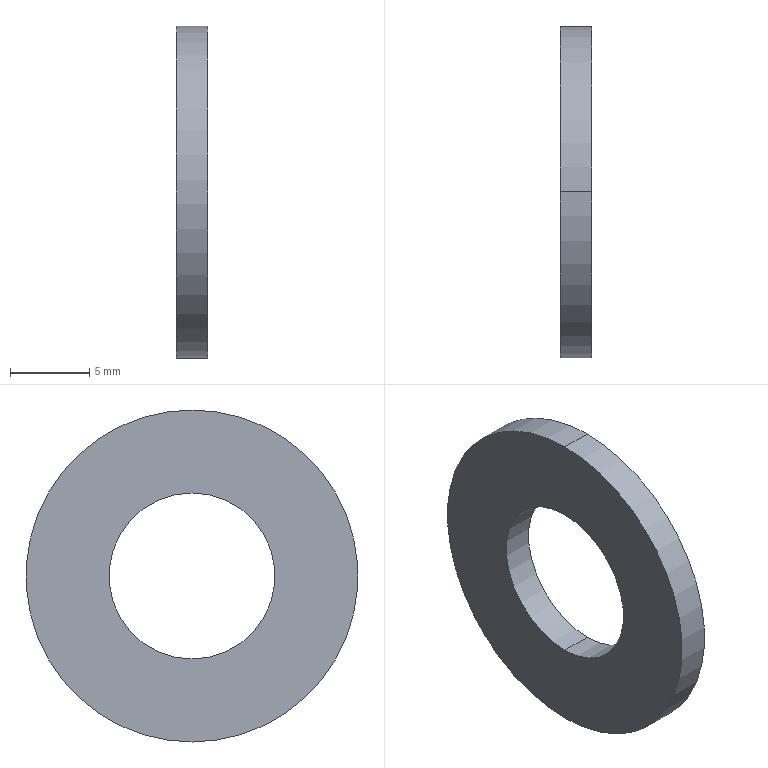Part | STEP file | 0229_316_SPWF10 | 1 solid | 6 faces | box 2 x 21 x 21 mm | volume 519.541 mm3 | cylinder 4 | plane 2 | commonest cylinder face diameters 10.5 x2 21 x2
STEP:
#1=CARTESIAN_POINT('',(0.,0.,0.));
#2=DIRECTION('',(0.,0.,1.));
#3=DIRECTION('',(1.,0.,0.));
#4=AXIS2_PLACEMENT_3D('',#1,#2,#3);
#5=CARTESIAN_POINT('',(-1.,0.,10.5));
#6=VERTEX_POINT('',#5);
#7=CARTESIAN_POINT('',(-1.,0.,-10.5));
#8=VERTEX_POINT('',#7);
#9=CARTESIAN_POINT('',(-1.,0.,0.));
#10=DIRECTION('',(-1.,0.,0.));
#11=DIRECTION('',(0.,0.,-1.));
#12=AXIS2_PLACEMENT_3D('',#9,#10,#11);
#13=CIRCLE('',#12,10.5);
#14=CARTESIAN_POINT('',(0.,0.,0.));
#15=DIRECTION('',(1.,0.,0.));
#16=DIRECTION('',(0.,0.,-1.));
#17=AXIS2_PLACEMENT_3D('',#14,#15,#16);
#18=CYLINDRICAL_SURFACE('',#17,10.5);
#19=CARTESIAN_POINT('',(6.283,-1.));
#20=DIRECTION('',(-1.,0.));
#21=VECTOR('',#20,1.);
#22=LINE('',#19,#21);
#23=(GEOMETRIC_REPRESENTATION_CONTEXT(2)PARAMETRIC_REPRESENTATION_CONTEXT()REPRESENTATION_CONTEXT('',''));
#24=DEFINITIONAL_REPRESENTATION('',(#22),#23);
#25=PCURVE('',#18,#24);
#26=CARTESIAN_POINT('',(-1.,7.875,0.));
#27=DIRECTION('',(-1.,0.,0.));
#28=DIRECTION('',(0.,0.,1.));
#29=AXIS2_PLACEMENT_3D('',#26,#27,#28);
#30=PLANE('',#29);
#31=CARTESIAN_POINT('',(0.,-7.875));
#32=DIRECTION('',(-1.,0.));
#33=AXIS2_PLACEMENT_2D('',#31,#32);
#34=CIRCLE('',#33,10.5);
#35=(GEOMETRIC_REPRESENTATION_CONTEXT(2)PARAMETRIC_REPRESENTATION_CONTEXT()REPRESENTATION_CONTEXT('',''));
#36=DEFINITIONAL_REPRESENTATION('',(#34),#35);
#37=PCURVE('',#30,#36);
#38=SURFACE_CURVE('',#13,(#25,#37),.PCURVE_S1.);
#39=EDGE_CURVE('',#6,#8,#38,.T.);
#40=ORIENTED_EDGE('',*,*,#39,.F.);
#41=CARTESIAN_POINT('',(1.,0.,10.5));
#42=VERTEX_POINT('',#41);
#43=CARTESIAN_POINT('',(0.,0.,10.5));
#44=DIRECTION('',(1.,0.,0.));
#45=VECTOR('',#44,1.);
#46=LINE('',#43,#45);
#47=CARTESIAN_POINT('',(3.142,0.));
#48=DIRECTION('',(0.,1.));
#49=VECTOR('',#48,1.);
#50=LINE('',#47,#49);
#51=(GEOMETRIC_REPRESENTATION_CONTEXT(2)PARAMETRIC_REPRESENTATION_CONTEXT()REPRESENTATION_CONTEXT('',''));
#52=DEFINITIONAL_REPRESENTATION('',(#50),#51);
#53=PCURVE('',#18,#52);
#54=CARTESIAN_POINT('',(0.,0.,0.));
#55=DIRECTION('',(1.,0.,0.));
#56=DIRECTION('',(0.,0.,-1.));
#57=AXIS2_PLACEMENT_3D('',#54,#55,#56);
#58=CYLINDRICAL_SURFACE('',#57,10.5);
#59=CARTESIAN_POINT('',(3.142,0.));
#60=DIRECTION('',(0.,1.));
#61=VECTOR('',#60,1.);
#62=LINE('',#59,#61);
#63=(GEOMETRIC_REPRESENTATION_CONTEXT(2)PARAMETRIC_REPRESENTATION_CONTEXT()REPRESENTATION_CONTEXT('',''));
#64=DEFINITIONAL_REPRESENTATION('',(#62),#63);
#65=PCURVE('',#58,#64);
#66=SURFACE_CURVE('',#46,(#53,#65),.PCURVE_S1.);
#67=EDGE_CURVE('',#6,#42,#66,.T.);
#68=ORIENTED_EDGE('',*,*,#67,.T.);
#69=CARTESIAN_POINT('',(1.,0.,-10.5));
#70=VERTEX_POINT('',#69);
#71=CARTESIAN_POINT('',(1.,0.,0.));
#72=DIRECTION('',(-1.,0.,0.));
#73=DIRECTION('',(0.,0.,-1.));
#74=AXIS2_PLACEMENT_3D('',#71,#72,#73);
#75=CIRCLE('',#74,10.5);
#76=CARTESIAN_POINT('',(6.283,1.));
#77=DIRECTION('',(-1.,0.));
#78=VECTOR('',#77,1.);
#79=LINE('',#76,#78);
#80=(GEOMETRIC_REPRESENTATION_CONTEXT(2)PARAMETRIC_REPRESENTATION_CONTEXT()REPRESENTATION_CONTEXT('',''));
#81=DEFINITIONAL_REPRESENTATION('',(#79),#80);
#82=PCURVE('',#18,#81);
#83=CARTESIAN_POINT('',(1.,7.875,0.));
#84=DIRECTION('',(1.,0.,0.));
#85=DIRECTION('',(0.,0.,-1.));
#86=AXIS2_PLACEMENT_3D('',#83,#84,#85);
#87=PLANE('',#86);
#88=CARTESIAN_POINT('',(10.5,-7.875));
#89=CARTESIAN_POINT('',(10.5,-26.062));
#90=CARTESIAN_POINT('',(-5.25,-16.968));
#91=CARTESIAN_POINT('',(-21.,-7.875));
#92=CARTESIAN_POINT('',(-5.25,1.218));
#93=CARTESIAN_POINT('',(10.5,10.312));
#94=CARTESIAN_POINT('',(10.5,-7.875));
#95=(BOUNDED_CURVE()B_SPLINE_CURVE(2,(#88,#89,#90,#91,#92,#93,#94),.UNSPECIFIED.,.T.,.F.)B_SPLINE_CURVE_WITH_KNOTS((1,2,2,2,2,1),(-2.094,0.,2.094,4.189,6.283,8.378),.UNSPECIFIED.)CURVE()GEOMETRIC_REPRESENTATION_ITEM()RATIONAL_B_SPLINE_CURVE((1.,0.5,1.,0.5,1.,0.5,1.))REPRESENTATION_ITEM(''));
#96=(GEOMETRIC_REPRESENTATION_CONTEXT(2)PARAMETRIC_REPRESENTATION_CONTEXT()REPRESENTATION_CONTEXT('',''));
#97=DEFINITIONAL_REPRESENTATION('',(#95),#96);
#98=PCURVE('',#87,#97);
#99=SURFACE_CURVE('',#75,(#82,#98),.PCURVE_S1.);
#100=EDGE_CURVE('',#42,#70,#99,.T.);
#101=ORIENTED_EDGE('',*,*,#100,.T.);
#102=CARTESIAN_POINT('',(0.,0.,-10.5));
#103=DIRECTION('',(1.,0.,0.));
#104=VECTOR('',#103,1.);
#105=LINE('',#102,#104);
#106=CARTESIAN_POINT('',(0.,0.));
#107=DIRECTION('',(0.,1.));
#108=VECTOR('',#107,1.);
#109=LINE('',#106,#108);
#110=(GEOMETRIC_REPRESENTATION_CONTEXT(2)PARAMETRIC_REPRESENTATION_CONTEXT()REPRESENTATION_CONTEXT('',''));
#111=DEFINITIONAL_REPRESENTATION('',(#109),#110);
#112=PCURVE('',#18,#111);
#113=CARTESIAN_POINT('',(6.283,0.));
#114=DIRECTION('',(0.,1.));
#115=VECTOR('',#114,1.);
#116=LINE('',#113,#115);
#117=(GEOMETRIC_REPRESENTATION_CONTEXT(2)PARAMETRIC_REPRESENTATION_CONTEXT()REPRESENTATION_CONTEXT('',''));
#118=DEFINITIONAL_REPRESENTATION('',(#116),#117);
#119=PCURVE('',#58,#118);
#120=SURFACE_CURVE('',#105,(#112,#119),.PCURVE_S1.);
#121=EDGE_CURVE('',#8,#70,#120,.T.);
#122=ORIENTED_EDGE('',*,*,#121,.F.);
#123=EDGE_LOOP('',(#40,#68,#101,#122));
#124=FACE_BOUND('',#123,.T.);
#125=ADVANCED_FACE('',(#124),#18,.T.);
#126=CARTESIAN_POINT('',(-1.,0.,-5.25));
#127=VERTEX_POINT('',#126);
#128=CARTESIAN_POINT('',(1.,0.,-5.25));
#129=VERTEX_POINT('',#128);
#130=CARTESIAN_POINT('',(0.,0.,-5.25));
#131=DIRECTION('',(1.,0.,0.));
#132=VECTOR('',#131,1.);
#133=LINE('',#130,#132);
#134=CARTESIAN_POINT('',(0.,0.,0.));
#135=DIRECTION('',(1.,0.,0.));
#136=DIRECTION('',(0.,0.,-1.));
#137=AXIS2_PLACEMENT_3D('',#134,#135,#136);
#138=CYLINDRICAL_SURFACE('',#137,5.25);
#139=CARTESIAN_POINT('',(6.283,0.));
#140=DIRECTION('',(0.,1.));
#141=VECTOR('',#140,1.);
#142=LINE('',#139,#141);
#143=(GEOMETRIC_REPRESENTATION_CONTEXT(2)PARAMETRIC_REPRESENTATION_CONTEXT()REPRESENTATION_CONTEXT('',''));
#144=DEFINITIONAL_REPRESENTATION('',(#142),#143);
#145=PCURVE('',#138,#144);
#146=CARTESIAN_POINT('',(0.,0.,0.));
#147=DIRECTION('',(1.,0.,0.));
#148=DIRECTION('',(0.,0.,-1.));
#149=AXIS2_PLACEMENT_3D('',#146,#147,#148);
#150=CYLINDRICAL_SURFACE('',#149,5.25);
#151=CARTESIAN_POINT('',(0.,0.));
#152=DIRECTION('',(0.,1.));
#153=VECTOR('',#152,1.);
#154=LINE('',#151,#153);
#155=(GEOMETRIC_REPRESENTATION_CONTEXT(2)PARAMETRIC_REPRESENTATION_CONTEXT()REPRESENTATION_CONTEXT('',''));
#156=DEFINITIONAL_REPRESENTATION('',(#154),#155);
#157=PCURVE('',#150,#156);
#158=SURFACE_CURVE('',#133,(#145,#157),.PCURVE_S1.);
#159=EDGE_CURVE('',#127,#129,#158,.T.);
#160=ORIENTED_EDGE('',*,*,#159,.T.);
#161=CARTESIAN_POINT('',(1.,0.,5.25));
#162=VERTEX_POINT('',#161);
#163=CARTESIAN_POINT('',(1.,0.,0.));
#164=DIRECTION('',(-1.,0.,0.));
#165=DIRECTION('',(0.,0.,-1.));
#166=AXIS2_PLACEMENT_3D('',#163,#164,#165);
#167=CIRCLE('',#166,5.25);
#168=CARTESIAN_POINT('',(6.283,1.));
#169=DIRECTION('',(-1.,0.));
#170=VECTOR('',#169,1.);
#171=LINE('',#168,#170);
#172=(GEOMETRIC_REPRESENTATION_CONTEXT(2)PARAMETRIC_REPRESENTATION_CONTEXT()REPRESENTATION_CONTEXT('',''));
#173=DEFINITIONAL_REPRESENTATION('',(#171),#172);
#174=PCURVE('',#138,#173);
#175=CARTESIAN_POINT('',(5.25,-7.875));
#176=CARTESIAN_POINT('',(5.25,-16.968));
#177=CARTESIAN_POINT('',(-2.625,-12.422));
#178=CARTESIAN_POINT('',(-10.5,-7.875));
#179=CARTESIAN_POINT('',(-2.625,-3.328));
#180=CARTESIAN_POINT('',(5.25,1.218));
#181=CARTESIAN_POINT('',(5.25,-7.875));
#182=(BOUNDED_CURVE()B_SPLINE_CURVE(2,(#175,#176,#177,#178,#179,#180,#181),.UNSPECIFIED.,.T.,.F.)B_SPLINE_CURVE_WITH_KNOTS((1,2,2,2,2,1),(-2.094,0.,2.094,4.189,6.283,8.378),.UNSPECIFIED.)CURVE()GEOMETRIC_REPRESENTATION_ITEM()RATIONAL_B_SPLINE_CURVE((1.,0.5,1.,0.5,1.,0.5,1.))REPRESENTATION_ITEM(''));
#183=(GEOMETRIC_REPRESENTATION_CONTEXT(2)PARAMETRIC_REPRESENTATION_CONTEXT()REPRESENTATION_CONTEXT('',''));
#184=DEFINITIONAL_REPRESENTATION('',(#182),#183);
#185=PCURVE('',#87,#184);
#186=SURFACE_CURVE('',#167,(#174,#185),.PCURVE_S1.);
#187=EDGE_CURVE('',#129,#162,#186,.T.);
#188=ORIENTED_EDGE('',*,*,#187,.T.);
#189=CARTESIAN_POINT('',(-1.,0.,5.25));
#190=VERTEX_POINT('',#189);
#191=CARTESIAN_POINT('',(0.,0.,5.25));
#192=DIRECTION('',(1.,0.,0.));
#193=VECTOR('',#192,1.);
#194=LINE('',#191,#193);
#195=CARTESIAN_POINT('',(3.142,0.));
#196=DIRECTION('',(0.,1.));
#197=VECTOR('',#196,1.);
#198=LINE('',#195,#197);
#199=(GEOMETRIC_REPRESENTATION_CONTEXT(2)PARAMETRIC_REPRESENTATION_CONTEXT()REPRESENTATION_CONTEXT('',''));
#200=DEFINITIONAL_REPRESENTATION('',(#198),#199);
#201=PCURVE('',#138,#200);
#202=CARTESIAN_POINT('',(3.142,0.));
#203=DIRECTION('',(0.,1.));
#204=VECTOR('',#203,1.);
#205=LINE('',#202,#204);
#206=(GEOMETRIC_REPRESENTATION_CONTEXT(2)PARAMETRIC_REPRESENTATION_CONTEXT()REPRESENTATION_CONTEXT('',''));
#207=DEFINITIONAL_REPRESENTATION('',(#205),#206);
#208=PCURVE('',#150,#207);
#209=SURFACE_CURVE('',#194,(#201,#208),.PCURVE_S1.);
#210=EDGE_CURVE('',#190,#162,#209,.T.);
#211=ORIENTED_EDGE('',*,*,#210,.F.);
#212=CARTESIAN_POINT('',(-1.,0.,0.));
#213=DIRECTION('',(1.,0.,0.));
#214=DIRECTION('',(0.,0.,-1.));
#215=AXIS2_PLACEMENT_3D('',#212,#213,#214);
#216=CIRCLE('',#215,5.25);
#217=CARTESIAN_POINT('',(0.,-1.));
#218=DIRECTION('',(1.,0.));
#219=VECTOR('',#218,1.);
#220=LINE('',#217,#219);
#221=(GEOMETRIC_REPRESENTATION_CONTEXT(2)PARAMETRIC_REPRESENTATION_CONTEXT()REPRESENTATION_CONTEXT('',''));
#222=DEFINITIONAL_REPRESENTATION('',(#220),#221);
#223=PCURVE('',#138,#222);
#224=CARTESIAN_POINT('',(-5.25,-7.875));
#225=CARTESIAN_POINT('',(-5.25,1.218));
#226=CARTESIAN_POINT('',(2.625,-3.328));
#227=CARTESIAN_POINT('',(10.5,-7.875));
#228=CARTESIAN_POINT('',(2.625,-12.422));
#229=CARTESIAN_POINT('',(-5.25,-16.968));
#230=CARTESIAN_POINT('',(-5.25,-7.875));
#231=(BOUNDED_CURVE()B_SPLINE_CURVE(2,(#224,#225,#226,#227,#228,#229,#230),.UNSPECIFIED.,.T.,.F.)B_SPLINE_CURVE_WITH_KNOTS((1,2,2,2,2,1),(-2.094,0.,2.094,4.189,6.283,8.378),.UNSPECIFIED.)CURVE()GEOMETRIC_REPRESENTATION_ITEM()RATIONAL_B_SPLINE_CURVE((1.,0.5,1.,0.5,1.,0.5,1.))REPRESENTATION_ITEM(''));
#232=(GEOMETRIC_REPRESENTATION_CONTEXT(2)PARAMETRIC_REPRESENTATION_CONTEXT()REPRESENTATION_CONTEXT('',''));
#233=DEFINITIONAL_REPRESENTATION('',(#231),#232);
#234=PCURVE('',#30,#233);
#235=SURFACE_CURVE('',#216,(#223,#234),.PCURVE_S1.);
#236=EDGE_CURVE('',#190,#127,#235,.T.);
#237=ORIENTED_EDGE('',*,*,#236,.T.);
#238=EDGE_LOOP('',(#160,#188,#211,#237));
#239=FACE_BOUND('',#238,.F.);
#240=ADVANCED_FACE('',(#239),#138,.F.);
#241=CARTESIAN_POINT('',(-1.,0.,0.));
#242=DIRECTION('',(-1.,0.,0.));
#243=DIRECTION('',(0.,0.,-1.));
#244=AXIS2_PLACEMENT_3D('',#241,#242,#243);
#245=CIRCLE('',#244,10.5);
#246=CARTESIAN_POINT('',(0.,-7.875));
#247=DIRECTION('',(-1.,0.));
#248=AXIS2_PLACEMENT_2D('',#246,#247);
#249=CIRCLE('',#248,10.5);
#250=(GEOMETRIC_REPRESENTATION_CONTEXT(2)PARAMETRIC_REPRESENTATION_CONTEXT()REPRESENTATION_CONTEXT('',''));
#251=DEFINITIONAL_REPRESENTATION('',(#249),#250);
#252=PCURVE('',#30,#251);
#253=CARTESIAN_POINT('',(6.283,-1.));
#254=DIRECTION('',(-1.,0.));
#255=VECTOR('',#254,1.);
#256=LINE('',#253,#255);
#257=(GEOMETRIC_REPRESENTATION_CONTEXT(2)PARAMETRIC_REPRESENTATION_CONTEXT()REPRESENTATION_CONTEXT('',''));
#258=DEFINITIONAL_REPRESENTATION('',(#256),#257);
#259=PCURVE('',#58,#258);
#260=SURFACE_CURVE('',#245,(#252,#259),.PCURVE_S1.);
#261=EDGE_CURVE('',#8,#6,#260,.T.);
#262=ORIENTED_EDGE('',*,*,#261,.T.);
#263=ORIENTED_EDGE('',*,*,#39,.T.);
#264=EDGE_LOOP('',(#262,#263));
#265=FACE_BOUND('',#264,.T.);
#266=CARTESIAN_POINT('',(-1.,0.,0.));
#267=DIRECTION('',(1.,0.,0.));
#268=DIRECTION('',(0.,0.,-1.));
#269=AXIS2_PLACEMENT_3D('',#266,#267,#268);
#270=CIRCLE('',#269,5.25);
#271=CARTESIAN_POINT('',(-5.25,-7.875));
#272=CARTESIAN_POINT('',(-5.25,1.218));
#273=CARTESIAN_POINT('',(2.625,-3.328));
#274=CARTESIAN_POINT('',(10.5,-7.875));
#275=CARTESIAN_POINT('',(2.625,-12.422));
#276=CARTESIAN_POINT('',(-5.25,-16.968));
#277=CARTESIAN_POINT('',(-5.25,-7.875));
#278=(BOUNDED_CURVE()B_SPLINE_CURVE(2,(#271,#272,#273,#274,#275,#276,#277),.UNSPECIFIED.,.T.,.F.)B_SPLINE_CURVE_WITH_KNOTS((1,2,2,2,2,1),(-2.094,0.,2.094,4.189,6.283,8.378),.UNSPECIFIED.)CURVE()GEOMETRIC_REPRESENTATION_ITEM()RATIONAL_B_SPLINE_CURVE((1.,0.5,1.,0.5,1.,0.5,1.))REPRESENTATION_ITEM(''));
#279=(GEOMETRIC_REPRESENTATION_CONTEXT(2)PARAMETRIC_REPRESENTATION_CONTEXT()REPRESENTATION_CONTEXT('',''));
#280=DEFINITIONAL_REPRESENTATION('',(#278),#279);
#281=PCURVE('',#30,#280);
#282=CARTESIAN_POINT('',(0.,-1.));
#283=DIRECTION('',(1.,0.));
#284=VECTOR('',#283,1.);
#285=LINE('',#282,#284);
#286=(GEOMETRIC_REPRESENTATION_CONTEXT(2)PARAMETRIC_REPRESENTATION_CONTEXT()REPRESENTATION_CONTEXT('',''));
#287=DEFINITIONAL_REPRESENTATION('',(#285),#286);
#288=PCURVE('',#150,#287);
#289=SURFACE_CURVE('',#270,(#281,#288),.PCURVE_S1.);
#290=EDGE_CURVE('',#127,#190,#289,.T.);
#291=ORIENTED_EDGE('',*,*,#290,.T.);
#292=ORIENTED_EDGE('',*,*,#236,.T.);
#293=EDGE_LOOP('',(#291,#292));
#294=FACE_BOUND('',#293,.T.);
#295=ADVANCED_FACE('',(#265,#294),#30,.T.);
#296=ORIENTED_EDGE('',*,*,#67,.F.);
#297=ORIENTED_EDGE('',*,*,#261,.F.);
#298=ORIENTED_EDGE('',*,*,#121,.T.);
#299=CARTESIAN_POINT('',(1.,0.,0.));
#300=DIRECTION('',(-1.,0.,0.));
#301=DIRECTION('',(0.,0.,-1.));
#302=AXIS2_PLACEMENT_3D('',#299,#300,#301);
#303=CIRCLE('',#302,10.5);
#304=CARTESIAN_POINT('',(6.283,1.));
#305=DIRECTION('',(-1.,0.));
#306=VECTOR('',#305,1.);
#307=LINE('',#304,#306);
#308=(GEOMETRIC_REPRESENTATION_CONTEXT(2)PARAMETRIC_REPRESENTATION_CONTEXT()REPRESENTATION_CONTEXT('',''));
#309=DEFINITIONAL_REPRESENTATION('',(#307),#308);
#310=PCURVE('',#58,#309);
#311=CARTESIAN_POINT('',(10.5,-7.875));
#312=CARTESIAN_POINT('',(10.5,-26.062));
#313=CARTESIAN_POINT('',(-5.25,-16.968));
#314=CARTESIAN_POINT('',(-21.,-7.875));
#315=CARTESIAN_POINT('',(-5.25,1.218));
#316=CARTESIAN_POINT('',(10.5,10.312));
#317=CARTESIAN_POINT('',(10.5,-7.875));
#318=(BOUNDED_CURVE()B_SPLINE_CURVE(2,(#311,#312,#313,#314,#315,#316,#317),.UNSPECIFIED.,.T.,.F.)B_SPLINE_CURVE_WITH_KNOTS((1,2,2,2,2,1),(-2.094,0.,2.094,4.189,6.283,8.378),.UNSPECIFIED.)CURVE()GEOMETRIC_REPRESENTATION_ITEM()RATIONAL_B_SPLINE_CURVE((1.,0.5,1.,0.5,1.,0.5,1.))REPRESENTATION_ITEM(''));
#319=(GEOMETRIC_REPRESENTATION_CONTEXT(2)PARAMETRIC_REPRESENTATION_CONTEXT()REPRESENTATION_CONTEXT('',''));
#320=DEFINITIONAL_REPRESENTATION('',(#318),#319);
#321=PCURVE('',#87,#320);
#322=SURFACE_CURVE('',#303,(#310,#321),.PCURVE_S1.);
#323=EDGE_CURVE('',#70,#42,#322,.T.);
#324=ORIENTED_EDGE('',*,*,#323,.T.);
#325=EDGE_LOOP('',(#296,#297,#298,#324));
#326=FACE_BOUND('',#325,.T.);
#327=ADVANCED_FACE('',(#326),#58,.T.);
#328=CARTESIAN_POINT('',(1.,0.,0.));
#329=DIRECTION('',(-1.,0.,0.));
#330=DIRECTION('',(0.,0.,-1.));
#331=AXIS2_PLACEMENT_3D('',#328,#329,#330);
#332=CIRCLE('',#331,5.25);
#333=CARTESIAN_POINT('',(6.283,1.));
#334=DIRECTION('',(-1.,0.));
#335=VECTOR('',#334,1.);
#336=LINE('',#333,#335);
#337=(GEOMETRIC_REPRESENTATION_CONTEXT(2)PARAMETRIC_REPRESENTATION_CONTEXT()REPRESENTATION_CONTEXT('',''));
#338=DEFINITIONAL_REPRESENTATION('',(#336),#337);
#339=PCURVE('',#150,#338);
#340=CARTESIAN_POINT('',(5.25,-7.875));
#341=CARTESIAN_POINT('',(5.25,-16.968));
#342=CARTESIAN_POINT('',(-2.625,-12.422));
#343=CARTESIAN_POINT('',(-10.5,-7.875));
#344=CARTESIAN_POINT('',(-2.625,-3.328));
#345=CARTESIAN_POINT('',(5.25,1.218));
#346=CARTESIAN_POINT('',(5.25,-7.875));
#347=(BOUNDED_CURVE()B_SPLINE_CURVE(2,(#340,#341,#342,#343,#344,#345,#346),.UNSPECIFIED.,.T.,.F.)B_SPLINE_CURVE_WITH_KNOTS((1,2,2,2,2,1),(-2.094,0.,2.094,4.189,6.283,8.378),.UNSPECIFIED.)CURVE()GEOMETRIC_REPRESENTATION_ITEM()RATIONAL_B_SPLINE_CURVE((1.,0.5,1.,0.5,1.,0.5,1.))REPRESENTATION_ITEM(''));
#348=(GEOMETRIC_REPRESENTATION_CONTEXT(2)PARAMETRIC_REPRESENTATION_CONTEXT()REPRESENTATION_CONTEXT('',''));
#349=DEFINITIONAL_REPRESENTATION('',(#347),#348);
#350=PCURVE('',#87,#349);
#351=SURFACE_CURVE('',#332,(#339,#350),.PCURVE_S1.);
#352=EDGE_CURVE('',#162,#129,#351,.T.);
#353=ORIENTED_EDGE('',*,*,#352,.T.);
#354=ORIENTED_EDGE('',*,*,#159,.F.);
#355=ORIENTED_EDGE('',*,*,#290,.T.);
#356=ORIENTED_EDGE('',*,*,#210,.T.);
#357=EDGE_LOOP('',(#353,#354,#355,#356));
#358=FACE_BOUND('',#357,.F.);
#359=ADVANCED_FACE('',(#358),#150,.F.);
#360=ORIENTED_EDGE('',*,*,#187,.T.);
#361=ORIENTED_EDGE('',*,*,#352,.T.);
#362=EDGE_LOOP('',(#360,#361));
#363=FACE_BOUND('',#362,.T.);
#364=ORIENTED_EDGE('',*,*,#323,.F.);
#365=ORIENTED_EDGE('',*,*,#100,.F.);
#366=EDGE_LOOP('',(#364,#365));
#367=FACE_BOUND('',#366,.T.);
#368=ADVANCED_FACE('',(#363,#367),#87,.T.);
#369=CLOSED_SHELL('',(#125,#240,#295,#327,#359,#368));
#370=MANIFOLD_SOLID_BREP('',#369);
#371=(LENGTH_UNIT()NAMED_UNIT(*)SI_UNIT(.MILLI.,.METRE.));
#372=UNCERTAINTY_MEASURE_WITH_UNIT(LENGTH_MEASURE(0.0000001),#371,'','');
#373=(NAMED_UNIT(*)PLANE_ANGLE_UNIT()SI_UNIT($,.RADIAN.));
#374=(NAMED_UNIT(*)SI_UNIT($,.STERADIAN.)SOLID_ANGLE_UNIT());
#375=(GEOMETRIC_REPRESENTATION_CONTEXT(3)GLOBAL_UNCERTAINTY_ASSIGNED_CONTEXT((#372))GLOBAL_UNIT_ASSIGNED_CONTEXT((#371,#373,#374))REPRESENTATION_CONTEXT('',''));
#376=ADVANCED_BREP_SHAPE_REPRESENTATION('',(#4,#370),#375);